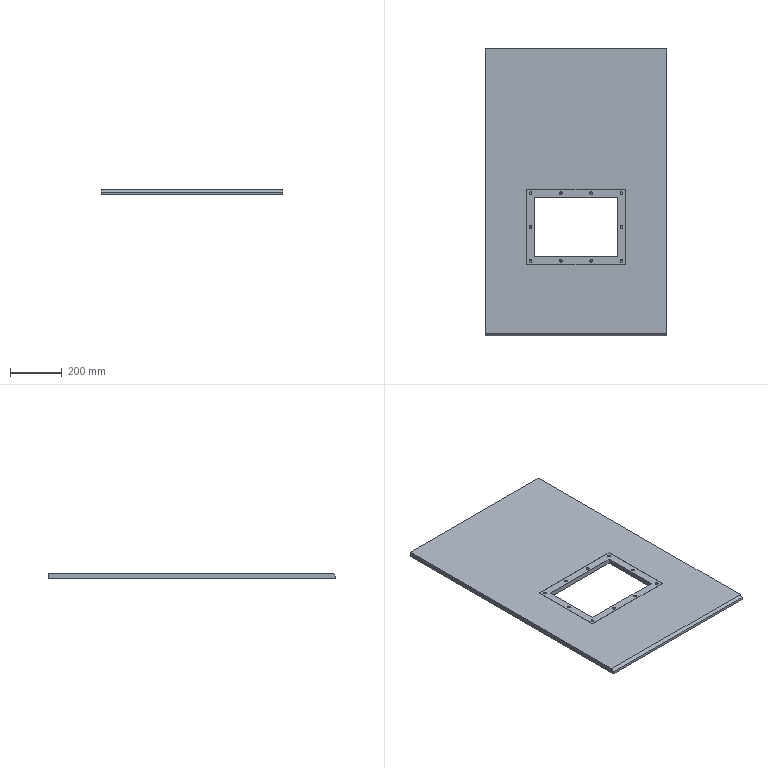Part | SolidWorks | features 3DProfileFeature 1, Chamfer 1, Extrusion 1, HoleWzd 1, ICE 1 | 1 solid | 56 faces | box 700 x 1110 x 20 mm | volume 13982805 mm3 | cylinder 20 | cone 20 | plane 16 | commonest cylinder face diameters 10.716 x20
STEP:
#1=CARTESIAN_POINT('',(169.642,550.,5.));
#2=VERTEX_POINT('',#1);
#3=CARTESIAN_POINT('',(180.358,550.,5.));
#4=VERTEX_POINT('',#3);
#5=CARTESIAN_POINT('',(175.,550.,5.));
#6=DIRECTION('',(0.,0.,1.));
#7=DIRECTION('',(1.,0.,0.));
#8=AXIS2_PLACEMENT_3D('',#5,#6,#7);
#9=CIRCLE('',#8,5.358);
#10=EDGE_CURVE('',#2,#4,#9,.T.);
#11=ORIENTED_EDGE('',*,*,#10,.F.);
#12=CARTESIAN_POINT('',(169.642,550.,19.));
#13=VERTEX_POINT('',#12);
#14=CARTESIAN_POINT('',(169.642,550.,19.));
#15=DIRECTION('',(0.,0.,1.));
#16=VECTOR('',#15,1000.);
#17=LINE('',#14,#16);
#18=EDGE_CURVE('',#2,#13,#17,.T.);
#19=ORIENTED_EDGE('',*,*,#18,.T.);
#20=CARTESIAN_POINT('',(180.358,550.,19.));
#21=VERTEX_POINT('',#20);
#22=CARTESIAN_POINT('',(175.,550.,19.));
#23=DIRECTION('',(0.,0.,1.));
#24=DIRECTION('',(1.,0.,0.));
#25=AXIS2_PLACEMENT_3D('',#22,#23,#24);
#26=CIRCLE('',#25,5.358);
#27=EDGE_CURVE('',#13,#21,#26,.T.);
#28=ORIENTED_EDGE('',*,*,#27,.T.);
#29=CARTESIAN_POINT('',(180.358,550.,19.));
#30=DIRECTION('',(0.,0.,1.));
#31=VECTOR('',#30,1000.);
#32=LINE('',#29,#31);
#33=EDGE_CURVE('',#4,#21,#32,.T.);
#34=ORIENTED_EDGE('',*,*,#33,.F.);
#35=EDGE_LOOP('',(#11,#19,#28,#34));
#36=FACE_OUTER_BOUND('',#35,.T.);
#37=CARTESIAN_POINT('',(175.,550.,19.));
#38=DIRECTION('',(0.,0.,1.));
#39=DIRECTION('',(1.,0.,0.));
#40=AXIS2_PLACEMENT_3D('',#37,#38,#39);
#41=CYLINDRICAL_SURFACE('',#40,5.358);
#42=ADVANCED_FACE('',(#36),#41,.F.);
#43=CARTESIAN_POINT('',(175.,550.,1.781));
#44=VERTEX_POINT('',#43);
#45=CARTESIAN_POINT('',(180.358,550.,5.));
#46=DIRECTION('',(0.8572,0.,0.515));
#47=VECTOR('',#46,1000.);
#48=LINE('',#45,#47);
#49=EDGE_CURVE('',#44,#4,#48,.T.);
#50=ORIENTED_EDGE('',*,*,#49,.F.);
#51=CARTESIAN_POINT('',(169.642,550.,5.));
#52=DIRECTION('',(-0.8572,0.,0.515));
#53=VECTOR('',#52,1000.);
#54=LINE('',#51,#53);
#55=EDGE_CURVE('',#44,#2,#54,.T.);
#56=ORIENTED_EDGE('',*,*,#55,.T.);
#57=ORIENTED_EDGE('',*,*,#10,.T.);
#58=EDGE_LOOP('',(#50,#56,#57));
#59=FACE_OUTER_BOUND('',#58,.T.);
#60=CARTESIAN_POINT('',(175.,550.,5.));
#61=DIRECTION('',(0.,0.,1.));
#62=DIRECTION('',(1.,0.,0.));
#63=AXIS2_PLACEMENT_3D('',#60,#61,#62);
#64=CONICAL_SURFACE('',#63,5.358,1.03);
#65=ADVANCED_FACE('',(#59),#64,.F.);
#66=CARTESIAN_POINT('',(286.142,550.,5.));
#67=VERTEX_POINT('',#66);
#68=CARTESIAN_POINT('',(296.858,550.,5.));
#69=VERTEX_POINT('',#68);
#70=CARTESIAN_POINT('',(291.5,550.,5.));
#71=DIRECTION('',(0.,0.,1.));
#72=DIRECTION('',(1.,0.,0.));
#73=AXIS2_PLACEMENT_3D('',#70,#71,#72);
#74=CIRCLE('',#73,5.358);
#75=EDGE_CURVE('',#67,#69,#74,.T.);
#76=ORIENTED_EDGE('',*,*,#75,.F.);
#77=CARTESIAN_POINT('',(286.142,550.,19.));
#78=VERTEX_POINT('',#77);
#79=CARTESIAN_POINT('',(286.142,550.,19.));
#80=DIRECTION('',(0.,0.,1.));
#81=VECTOR('',#80,1000.);
#82=LINE('',#79,#81);
#83=EDGE_CURVE('',#67,#78,#82,.T.);
#84=ORIENTED_EDGE('',*,*,#83,.T.);
#85=CARTESIAN_POINT('',(296.858,550.,19.));
#86=VERTEX_POINT('',#85);
#87=CARTESIAN_POINT('',(291.5,550.,19.));
#88=DIRECTION('',(0.,0.,1.));
#89=DIRECTION('',(1.,0.,0.));
#90=AXIS2_PLACEMENT_3D('',#87,#88,#89);
#91=CIRCLE('',#90,5.358);
#92=EDGE_CURVE('',#78,#86,#91,.T.);
#93=ORIENTED_EDGE('',*,*,#92,.T.);
#94=CARTESIAN_POINT('',(296.858,550.,19.));
#95=DIRECTION('',(0.,0.,1.));
#96=VECTOR('',#95,1000.);
#97=LINE('',#94,#96);
#98=EDGE_CURVE('',#69,#86,#97,.T.);
#99=ORIENTED_EDGE('',*,*,#98,.F.);
#100=EDGE_LOOP('',(#76,#84,#93,#99));
#101=FACE_OUTER_BOUND('',#100,.T.);
#102=CARTESIAN_POINT('',(291.5,550.,19.));
#103=DIRECTION('',(0.,0.,1.));
#104=DIRECTION('',(1.,0.,0.));
#105=AXIS2_PLACEMENT_3D('',#102,#103,#104);
#106=CYLINDRICAL_SURFACE('',#105,5.358);
#107=ADVANCED_FACE('',(#101),#106,.F.);
#108=CARTESIAN_POINT('',(291.5,550.,1.781));
#109=VERTEX_POINT('',#108);
#110=CARTESIAN_POINT('',(296.858,550.,5.));
#111=DIRECTION('',(0.8572,0.,0.515));
#112=VECTOR('',#111,1000.);
#113=LINE('',#110,#112);
#114=EDGE_CURVE('',#109,#69,#113,.T.);
#115=ORIENTED_EDGE('',*,*,#114,.F.);
#116=CARTESIAN_POINT('',(286.142,550.,5.));
#117=DIRECTION('',(-0.8572,0.,0.515));
#118=VECTOR('',#117,1000.);
#119=LINE('',#116,#118);
#120=EDGE_CURVE('',#109,#67,#119,.T.);
#121=ORIENTED_EDGE('',*,*,#120,.T.);
#122=ORIENTED_EDGE('',*,*,#75,.T.);
#123=EDGE_LOOP('',(#115,#121,#122));
#124=FACE_OUTER_BOUND('',#123,.T.);
#125=CARTESIAN_POINT('',(291.5,550.,5.));
#126=DIRECTION('',(0.,0.,1.));
#127=DIRECTION('',(1.,0.,0.));
#128=AXIS2_PLACEMENT_3D('',#125,#126,#127);
#129=CONICAL_SURFACE('',#128,5.358,1.03);
#130=ADVANCED_FACE('',(#124),#129,.F.);
#131=CARTESIAN_POINT('',(403.142,550.,5.));
#132=VERTEX_POINT('',#131);
#133=CARTESIAN_POINT('',(413.858,550.,5.));
#134=VERTEX_POINT('',#133);
#135=CARTESIAN_POINT('',(408.5,550.,5.));
#136=DIRECTION('',(0.,0.,1.));
#137=DIRECTION('',(1.,0.,0.));
#138=AXIS2_PLACEMENT_3D('',#135,#136,#137);
#139=CIRCLE('',#138,5.358);
#140=EDGE_CURVE('',#132,#134,#139,.T.);
#141=ORIENTED_EDGE('',*,*,#140,.F.);
#142=CARTESIAN_POINT('',(403.142,550.,19.));
#143=VERTEX_POINT('',#142);
#144=CARTESIAN_POINT('',(403.142,550.,19.));
#145=DIRECTION('',(0.,0.,1.));
#146=VECTOR('',#145,1000.);
#147=LINE('',#144,#146);
#148=EDGE_CURVE('',#132,#143,#147,.T.);
#149=ORIENTED_EDGE('',*,*,#148,.T.);
#150=CARTESIAN_POINT('',(413.858,550.,19.));
#151=VERTEX_POINT('',#150);
#152=CARTESIAN_POINT('',(408.5,550.,19.));
#153=DIRECTION('',(0.,0.,1.));
#154=DIRECTION('',(1.,0.,0.));
#155=AXIS2_PLACEMENT_3D('',#152,#153,#154);
#156=CIRCLE('',#155,5.358);
#157=EDGE_CURVE('',#143,#151,#156,.T.);
#158=ORIENTED_EDGE('',*,*,#157,.T.);
#159=CARTESIAN_POINT('',(413.858,550.,19.));
#160=DIRECTION('',(0.,0.,1.));
#161=VECTOR('',#160,1000.);
#162=LINE('',#159,#161);
#163=EDGE_CURVE('',#134,#151,#162,.T.);
#164=ORIENTED_EDGE('',*,*,#163,.F.);
#165=EDGE_LOOP('',(#141,#149,#158,#164));
#166=FACE_OUTER_BOUND('',#165,.T.);
#167=CARTESIAN_POINT('',(408.5,550.,19.));
#168=DIRECTION('',(0.,0.,1.));
#169=DIRECTION('',(1.,0.,0.));
#170=AXIS2_PLACEMENT_3D('',#167,#168,#169);
#171=CYLINDRICAL_SURFACE('',#170,5.358);
#172=ADVANCED_FACE('',(#166),#171,.F.);
#173=CARTESIAN_POINT('',(408.5,550.,1.781));
#174=VERTEX_POINT('',#173);
#175=CARTESIAN_POINT('',(413.858,550.,5.));
#176=DIRECTION('',(0.8572,0.,0.515));
#177=VECTOR('',#176,1000.);
#178=LINE('',#175,#177);
#179=EDGE_CURVE('',#174,#134,#178,.T.);
#180=ORIENTED_EDGE('',*,*,#179,.F.);
#181=CARTESIAN_POINT('',(403.142,550.,5.));
#182=DIRECTION('',(-0.8572,0.,0.515));
#183=VECTOR('',#182,1000.);
#184=LINE('',#181,#183);
#185=EDGE_CURVE('',#174,#132,#184,.T.);
#186=ORIENTED_EDGE('',*,*,#185,.T.);
#187=ORIENTED_EDGE('',*,*,#140,.T.);
#188=EDGE_LOOP('',(#180,#186,#187));
#189=FACE_OUTER_BOUND('',#188,.T.);
#190=CARTESIAN_POINT('',(408.5,550.,5.));
#191=DIRECTION('',(0.,0.,1.));
#192=DIRECTION('',(1.,0.,0.));
#193=AXIS2_PLACEMENT_3D('',#190,#191,#192);
#194=CONICAL_SURFACE('',#193,5.358,1.03);
#195=ADVANCED_FACE('',(#189),#194,.F.);
#196=CARTESIAN_POINT('',(519.642,550.,5.));
#197=VERTEX_POINT('',#196);
#198=CARTESIAN_POINT('',(530.358,550.,5.));
#199=VERTEX_POINT('',#198);
#200=CARTESIAN_POINT('',(525.,550.,5.));
#201=DIRECTION('',(0.,0.,1.));
#202=DIRECTION('',(1.,0.,0.));
#203=AXIS2_PLACEMENT_3D('',#200,#201,#202);
#204=CIRCLE('',#203,5.358);
#205=EDGE_CURVE('',#197,#199,#204,.T.);
#206=ORIENTED_EDGE('',*,*,#205,.F.);
#207=CARTESIAN_POINT('',(519.642,550.,19.));
#208=VERTEX_POINT('',#207);
#209=CARTESIAN_POINT('',(519.642,550.,19.));
#210=DIRECTION('',(0.,0.,1.));
#211=VECTOR('',#210,1000.);
#212=LINE('',#209,#211);
#213=EDGE_CURVE('',#197,#208,#212,.T.);
#214=ORIENTED_EDGE('',*,*,#213,.T.);
#215=CARTESIAN_POINT('',(530.358,550.,19.));
#216=VERTEX_POINT('',#215);
#217=CARTESIAN_POINT('',(525.,550.,19.));
#218=DIRECTION('',(0.,0.,1.));
#219=DIRECTION('',(1.,0.,0.));
#220=AXIS2_PLACEMENT_3D('',#217,#218,#219);
#221=CIRCLE('',#220,5.358);
#222=EDGE_CURVE('',#208,#216,#221,.T.);
#223=ORIENTED_EDGE('',*,*,#222,.T.);
#224=CARTESIAN_POINT('',(530.358,550.,19.));
#225=DIRECTION('',(0.,0.,1.));
#226=VECTOR('',#225,1000.);
#227=LINE('',#224,#226);
#228=EDGE_CURVE('',#199,#216,#227,.T.);
#229=ORIENTED_EDGE('',*,*,#228,.F.);
#230=EDGE_LOOP('',(#206,#214,#223,#229));
#231=FACE_OUTER_BOUND('',#230,.T.);
#232=CARTESIAN_POINT('',(525.,550.,19.));
#233=DIRECTION('',(0.,0.,1.));
#234=DIRECTION('',(1.,0.,0.));
#235=AXIS2_PLACEMENT_3D('',#232,#233,#234);
#236=CYLINDRICAL_SURFACE('',#235,5.358);
#237=ADVANCED_FACE('',(#231),#236,.F.);
#238=CARTESIAN_POINT('',(525.,550.,1.781));
#239=VERTEX_POINT('',#238);
#240=CARTESIAN_POINT('',(530.358,550.,5.));
#241=DIRECTION('',(0.8572,0.,0.515));
#242=VECTOR('',#241,1000.);
#243=LINE('',#240,#242);
#244=EDGE_CURVE('',#239,#199,#243,.T.);
#245=ORIENTED_EDGE('',*,*,#244,.F.);
#246=CARTESIAN_POINT('',(519.642,550.,5.));
#247=DIRECTION('',(-0.8572,0.,0.515));
#248=VECTOR('',#247,1000.);
#249=LINE('',#246,#248);
#250=EDGE_CURVE('',#239,#197,#249,.T.);
#251=ORIENTED_EDGE('',*,*,#250,.T.);
#252=ORIENTED_EDGE('',*,*,#205,.T.);
#253=EDGE_LOOP('',(#245,#251,#252));
#254=FACE_OUTER_BOUND('',#253,.T.);
#255=CARTESIAN_POINT('',(525.,550.,5.));
#256=DIRECTION('',(0.,0.,1.));
#257=DIRECTION('',(1.,0.,0.));
#258=AXIS2_PLACEMENT_3D('',#255,#256,#257);
#259=CONICAL_SURFACE('',#258,5.358,1.03);
#260=ADVANCED_FACE('',(#254),#259,.F.);
#261=CARTESIAN_POINT('',(519.642,420.,5.));
#262=VERTEX_POINT('',#261);
#263=CARTESIAN_POINT('',(530.358,420.,5.));
#264=VERTEX_POINT('',#263);
#265=CARTESIAN_POINT('',(525.,420.,5.));
#266=DIRECTION('',(0.,0.,1.));
#267=DIRECTION('',(1.,0.,0.));
#268=AXIS2_PLACEMENT_3D('',#265,#266,#267);
#269=CIRCLE('',#268,5.358);
#270=EDGE_CURVE('',#262,#264,#269,.T.);
#271=ORIENTED_EDGE('',*,*,#270,.F.);
#272=CARTESIAN_POINT('',(519.642,420.,19.));
#273=VERTEX_POINT('',#272);
#274=CARTESIAN_POINT('',(519.642,420.,19.));
#275=DIRECTION('',(0.,0.,1.));
#276=VECTOR('',#275,1000.);
#277=LINE('',#274,#276);
#278=EDGE_CURVE('',#262,#273,#277,.T.);
#279=ORIENTED_EDGE('',*,*,#278,.T.);
#280=CARTESIAN_POINT('',(530.358,420.,19.));
#281=VERTEX_POINT('',#280);
#282=CARTESIAN_POINT('',(525.,420.,19.));
#283=DIRECTION('',(0.,0.,1.));
#284=DIRECTION('',(1.,0.,0.));
#285=AXIS2_PLACEMENT_3D('',#282,#283,#284);
#286=CIRCLE('',#285,5.358);
#287=EDGE_CURVE('',#273,#281,#286,.T.);
#288=ORIENTED_EDGE('',*,*,#287,.T.);
#289=CARTESIAN_POINT('',(530.358,420.,19.));
#290=DIRECTION('',(0.,0.,1.));
#291=VECTOR('',#290,1000.);
#292=LINE('',#289,#291);
#293=EDGE_CURVE('',#264,#281,#292,.T.);
#294=ORIENTED_EDGE('',*,*,#293,.F.);
#295=EDGE_LOOP('',(#271,#279,#288,#294));
#296=FACE_OUTER_BOUND('',#295,.T.);
#297=CARTESIAN_POINT('',(525.,420.,19.));
#298=DIRECTION('',(0.,0.,1.));
#299=DIRECTION('',(1.,0.,0.));
#300=AXIS2_PLACEMENT_3D('',#297,#298,#299);
#301=CYLINDRICAL_SURFACE('',#300,5.358);
#302=ADVANCED_FACE('',(#296),#301,.F.);
#303=CARTESIAN_POINT('',(525.,420.,1.781));
#304=VERTEX_POINT('',#303);
#305=CARTESIAN_POINT('',(530.358,420.,5.));
#306=DIRECTION('',(0.8572,0.,0.515));
#307=VECTOR('',#306,1000.);
#308=LINE('',#305,#307);
#309=EDGE_CURVE('',#304,#264,#308,.T.);
#310=ORIENTED_EDGE('',*,*,#309,.F.);
#311=CARTESIAN_POINT('',(519.642,420.,5.));
#312=DIRECTION('',(-0.8572,0.,0.515));
#313=VECTOR('',#312,1000.);
#314=LINE('',#311,#313);
#315=EDGE_CURVE('',#304,#262,#314,.T.);
#316=ORIENTED_EDGE('',*,*,#315,.T.);
#317=ORIENTED_EDGE('',*,*,#270,.T.);
#318=EDGE_LOOP('',(#310,#316,#317));
#319=FACE_OUTER_BOUND('',#318,.T.);
#320=CARTESIAN_POINT('',(525.,420.,5.));
#321=DIRECTION('',(0.,0.,1.));
#322=DIRECTION('',(1.,0.,0.));
#323=AXIS2_PLACEMENT_3D('',#320,#321,#322);
#324=CONICAL_SURFACE('',#323,5.358,1.03);
#325=ADVANCED_FACE('',(#319),#324,.F.);
#326=CARTESIAN_POINT('',(519.642,290.,5.));
#327=VERTEX_POINT('',#326);
#328=CARTESIAN_POINT('',(530.358,290.,5.));
#329=VERTEX_POINT('',#328);
#330=CARTESIAN_POINT('',(525.,290.,5.));
#331=DIRECTION('',(0.,0.,1.));
#332=DIRECTION('',(1.,0.,0.));
#333=AXIS2_PLACEMENT_3D('',#330,#331,#332);
#334=CIRCLE('',#333,5.358);
#335=EDGE_CURVE('',#327,#329,#334,.T.);
#336=ORIENTED_EDGE('',*,*,#335,.F.);
#337=CARTESIAN_POINT('',(519.642,290.,19.));
#338=VERTEX_POINT('',#337);
#339=CARTESIAN_POINT('',(519.642,290.,19.));
#340=DIRECTION('',(0.,0.,1.));
#341=VECTOR('',#340,1000.);
#342=LINE('',#339,#341);
#343=EDGE_CURVE('',#327,#338,#342,.T.);
#344=ORIENTED_EDGE('',*,*,#343,.T.);
#345=CARTESIAN_POINT('',(530.358,290.,19.));
#346=VERTEX_POINT('',#345);
#347=CARTESIAN_POINT('',(525.,290.,19.));
#348=DIRECTION('',(0.,0.,1.));
#349=DIRECTION('',(1.,0.,0.));
#350=AXIS2_PLACEMENT_3D('',#347,#348,#349);
#351=CIRCLE('',#350,5.358);
#352=EDGE_CURVE('',#338,#346,#351,.T.);
#353=ORIENTED_EDGE('',*,*,#352,.T.);
#354=CARTESIAN_POINT('',(530.358,290.,19.));
#355=DIRECTION('',(0.,0.,1.));
#356=VECTOR('',#355,1000.);
#357=LINE('',#354,#356);
#358=EDGE_CURVE('',#329,#346,#357,.T.);
#359=ORIENTED_EDGE('',*,*,#358,.F.);
#360=EDGE_LOOP('',(#336,#344,#353,#359));
#361=FACE_OUTER_BOUND('',#360,.T.);
#362=CARTESIAN_POINT('',(525.,290.,19.));
#363=DIRECTION('',(0.,0.,1.));
#364=DIRECTION('',(1.,0.,0.));
#365=AXIS2_PLACEMENT_3D('',#362,#363,#364);
#366=CYLINDRICAL_SURFACE('',#365,5.358);
#367=ADVANCED_FACE('',(#361),#366,.F.);
#368=CARTESIAN_POINT('',(525.,290.,1.781));
#369=VERTEX_POINT('',#368);
#370=CARTESIAN_POINT('',(530.358,290.,5.));
#371=DIRECTION('',(0.8572,0.,0.515));
#372=VECTOR('',#371,1000.);
#373=LINE('',#370,#372);
#374=EDGE_CURVE('',#369,#329,#373,.T.);
#375=ORIENTED_EDGE('',*,*,#374,.F.);
#376=CARTESIAN_POINT('',(519.642,290.,5.));
#377=DIRECTION('',(-0.8572,0.,0.515));
#378=VECTOR('',#377,1000.);
#379=LINE('',#376,#378);
#380=EDGE_CURVE('',#369,#327,#379,.T.);
#381=ORIENTED_EDGE('',*,*,#380,.T.);
#382=ORIENTED_EDGE('',*,*,#335,.T.);
#383=EDGE_LOOP('',(#375,#381,#382));
#384=FACE_OUTER_BOUND('',#383,.T.);
#385=CARTESIAN_POINT('',(525.,290.,5.));
#386=DIRECTION('',(0.,0.,1.));
#387=DIRECTION('',(1.,0.,0.));
#388=AXIS2_PLACEMENT_3D('',#385,#386,#387);
#389=CONICAL_SURFACE('',#388,5.358,1.03);
#390=ADVANCED_FACE('',(#384),#389,.F.);
#391=CARTESIAN_POINT('',(403.142,290.,5.));
#392=VERTEX_POINT('',#391);
#393=CARTESIAN_POINT('',(413.858,290.,5.));
#394=VERTEX_POINT('',#393);
#395=CARTESIAN_POINT('',(408.5,290.,5.));
#396=DIRECTION('',(0.,0.,1.));
#397=DIRECTION('',(1.,0.,0.));
#398=AXIS2_PLACEMENT_3D('',#395,#396,#397);
#399=CIRCLE('',#398,5.358);
#400=EDGE_CURVE('',#392,#394,#399,.T.);
#401=ORIENTED_EDGE('',*,*,#400,.F.);
#402=CARTESIAN_POINT('',(403.142,290.,19.));
#403=VERTEX_POINT('',#402);
#404=CARTESIAN_POINT('',(403.142,290.,19.));
#405=DIRECTION('',(0.,0.,1.));
#406=VECTOR('',#405,1000.);
#407=LINE('',#404,#406);
#408=EDGE_CURVE('',#392,#403,#407,.T.);
#409=ORIENTED_EDGE('',*,*,#408,.T.);
#410=CARTESIAN_POINT('',(413.858,290.,19.));
#411=VERTEX_POINT('',#410);
#412=CARTESIAN_POINT('',(408.5,290.,19.));
#413=DIRECTION('',(0.,0.,1.));
#414=DIRECTION('',(1.,0.,0.));
#415=AXIS2_PLACEMENT_3D('',#412,#413,#414);
#416=CIRCLE('',#415,5.358);
#417=EDGE_CURVE('',#403,#411,#416,.T.);
#418=ORIENTED_EDGE('',*,*,#417,.T.);
#419=CARTESIAN_POINT('',(413.858,290.,19.));
#420=DIRECTION('',(0.,0.,1.));
#421=VECTOR('',#420,1000.);
#422=LINE('',#419,#421);
#423=EDGE_CURVE('',#394,#411,#422,.T.);
#424=ORIENTED_EDGE('',*,*,#423,.F.);
#425=EDGE_LOOP('',(#401,#409,#418,#424));
#426=FACE_OUTER_BOUND('',#425,.T.);
#427=CARTESIAN_POINT('',(408.5,290.,19.));
#428=DIRECTION('',(0.,0.,1.));
#429=DIRECTION('',(1.,0.,0.));
#430=AXIS2_PLACEMENT_3D('',#427,#428,#429);
#431=CYLINDRICAL_SURFACE('',#430,5.358);
#432=ADVANCED_FACE('',(#426),#431,.F.);
#433=CARTESIAN_POINT('',(408.5,290.,1.781));
#434=VERTEX_POINT('',#433);
#435=CARTESIAN_POINT('',(413.858,290.,5.));
#436=DIRECTION('',(0.8572,0.,0.515));
#437=VECTOR('',#436,1000.);
#438=LINE('',#435,#437);
#439=EDGE_CURVE('',#434,#394,#438,.T.);
#440=ORIENTED_EDGE('',*,*,#439,.F.);
#441=CARTESIAN_POINT('',(403.142,290.,5.));
#442=DIRECTION('',(-0.8572,0.,0.515));
#443=VECTOR('',#442,1000.);
#444=LINE('',#441,#443);
#445=EDGE_CURVE('',#434,#392,#444,.T.);
#446=ORIENTED_EDGE('',*,*,#445,.T.);
#447=ORIENTED_EDGE('',*,*,#400,.T.);
#448=EDGE_LOOP('',(#440,#446,#447));
#449=FACE_OUTER_BOUND('',#448,.T.);
#450=CARTESIAN_POINT('',(408.5,290.,5.));
#451=DIRECTION('',(0.,0.,1.));
#452=DIRECTION('',(1.,0.,0.));
#453=AXIS2_PLACEMENT_3D('',#450,#451,#452);
#454=CONICAL_SURFACE('',#453,5.358,1.03);
#455=ADVANCED_FACE('',(#449),#454,.F.);
#456=CARTESIAN_POINT('',(286.142,290.,5.));
#457=VERTEX_POINT('',#456);
#458=CARTESIAN_POINT('',(296.858,290.,5.));
#459=VERTEX_POINT('',#458);
#460=CARTESIAN_POINT('',(291.5,290.,5.));
#461=DIRECTION('',(0.,0.,1.));
#462=DIRECTION('',(1.,0.,0.));
#463=AXIS2_PLACEMENT_3D('',#460,#461,#462);
#464=CIRCLE('',#463,5.358);
#465=EDGE_CURVE('',#457,#459,#464,.T.);
#466=ORIENTED_EDGE('',*,*,#465,.F.);
#467=CARTESIAN_POINT('',(286.142,290.,19.));
#468=VERTEX_POINT('',#467);
#469=CARTESIAN_POINT('',(286.142,290.,19.));
#470=DIRECTION('',(0.,0.,1.));
#471=VECTOR('',#470,1000.);
#472=LINE('',#469,#471);
#473=EDGE_CURVE('',#457,#468,#472,.T.);
#474=ORIENTED_EDGE('',*,*,#473,.T.);
#475=CARTESIAN_POINT('',(296.858,290.,19.));
#476=VERTEX_POINT('',#475);
#477=CARTESIAN_POINT('',(291.5,290.,19.));
#478=DIRECTION('',(0.,0.,1.));
#479=DIRECTION('',(1.,0.,0.));
#480=AXIS2_PLACEMENT_3D('',#477,#478,#479);
#481=CIRCLE('',#480,5.358);
#482=EDGE_CURVE('',#468,#476,#481,.T.);
#483=ORIENTED_EDGE('',*,*,#482,.T.);
#484=CARTESIAN_POINT('',(296.858,290.,19.));
#485=DIRECTION('',(0.,0.,1.));
#486=VECTOR('',#485,1000.);
#487=LINE('',#484,#486);
#488=EDGE_CURVE('',#459,#476,#487,.T.);
#489=ORIENTED_EDGE('',*,*,#488,.F.);
#490=EDGE_LOOP('',(#466,#474,#483,#489));
#491=FACE_OUTER_BOUND('',#490,.T.);
#492=CARTESIAN_POINT('',(291.5,290.,19.));
#493=DIRECTION('',(0.,0.,1.));
#494=DIRECTION('',(1.,0.,0.));
#495=AXIS2_PLACEMENT_3D('',#492,#493,#494);
#496=CYLINDRICAL_SURFACE('',#495,5.358);
#497=ADVANCED_FACE('',(#491),#496,.F.);
#498=CARTESIAN_POINT('',(291.5,290.,1.781));
#499=VERTEX_POINT('',#498);
#500=CARTESIAN_POINT('',(296.858,290.,5.));
#501=DIRECTION('',(0.8572,0.,0.515));
#502=VECTOR('',#501,1000.);
#503=LINE('',#500,#502);
#504=EDGE_CURVE('',#499,#459,#503,.T.);
#505=ORIENTED_EDGE('',*,*,#504,.F.);
#506=CARTESIAN_POINT('',(286.142,290.,5.));
#507=DIRECTION('',(-0.8572,0.,0.515));
#508=VECTOR('',#507,1000.);
#509=LINE('',#506,#508);
#510=EDGE_CURVE('',#499,#457,#509,.T.);
#511=ORIENTED_EDGE('',*,*,#510,.T.);
#512=ORIENTED_EDGE('',*,*,#465,.T.);
#513=EDGE_LOOP('',(#505,#511,#512));
#514=FACE_OUTER_BOUND('',#513,.T.);
#515=CARTESIAN_POINT('',(291.5,290.,5.));
#516=DIRECTION('',(0.,0.,1.));
#517=DIRECTION('',(1.,0.,0.));
#518=AXIS2_PLACEMENT_3D('',#515,#516,#517);
#519=CONICAL_SURFACE('',#518,5.358,1.03);
#520=ADVANCED_FACE('',(#514),#519,.F.);
#521=CARTESIAN_POINT('',(169.642,290.,5.));
#522=VERTEX_POINT('',#521);
#523=CARTESIAN_POINT('',(180.358,290.,5.));
#524=VERTEX_POINT('',#523);
#525=CARTESIAN_POINT('',(175.,290.,5.));
#526=DIRECTION('',(0.,0.,1.));
#527=DIRECTION('',(1.,0.,0.));
#528=AXIS2_PLACEMENT_3D('',#525,#526,#527);
#529=CIRCLE('',#528,5.358);
#530=EDGE_CURVE('',#522,#524,#529,.T.);
#531=ORIENTED_EDGE('',*,*,#530,.F.);
#532=CARTESIAN_POINT('',(169.642,290.,19.));
#533=VERTEX_POINT('',#532);
#534=CARTESIAN_POINT('',(169.642,290.,19.));
#535=DIRECTION('',(0.,0.,1.));
#536=VECTOR('',#535,1000.);
#537=LINE('',#534,#536);
#538=EDGE_CURVE('',#522,#533,#537,.T.);
#539=ORIENTED_EDGE('',*,*,#538,.T.);
#540=CARTESIAN_POINT('',(180.358,290.,19.));
#541=VERTEX_POINT('',#540);
#542=CARTESIAN_POINT('',(175.,290.,19.));
#543=DIRECTION('',(0.,0.,1.));
#544=DIRECTION('',(1.,0.,0.));
#545=AXIS2_PLACEMENT_3D('',#542,#543,#544);
#546=CIRCLE('',#545,5.358);
#547=EDGE_CURVE('',#533,#541,#546,.T.);
#548=ORIENTED_EDGE('',*,*,#547,.T.);
#549=CARTESIAN_POINT('',(180.358,290.,19.));
#550=DIRECTION('',(0.,0.,1.));
#551=VECTOR('',#550,1000.);
#552=LINE('',#549,#551);
#553=EDGE_CURVE('',#524,#541,#552,.T.);
#554=ORIENTED_EDGE('',*,*,#553,.F.);
#555=EDGE_LOOP('',(#531,#539,#548,#554));
#556=FACE_OUTER_BOUND('',#555,.T.);
#557=CARTESIAN_POINT('',(175.,290.,19.));
#558=DIRECTION('',(0.,0.,1.));
#559=DIRECTION('',(1.,0.,0.));
#560=AXIS2_PLACEMENT_3D('',#557,#558,#559);
#561=CYLINDRICAL_SURFACE('',#560,5.358);
#562=ADVANCED_FACE('',(#556),#561,.F.);
#563=CARTESIAN_POINT('',(175.,290.,1.781));
#564=VERTEX_POINT('',#563);
#565=CARTESIAN_POINT('',(180.358,290.,5.));
#566=DIRECTION('',(0.8572,0.,0.515));
#567=VECTOR('',#566,1000.);
#568=LINE('',#565,#567);
#569=EDGE_CURVE('',#564,#524,#568,.T.);
#570=ORIENTED_EDGE('',*,*,#569,.F.);
#571=CARTESIAN_POINT('',(169.642,290.,5.));
#572=DIRECTION('',(-0.8572,0.,0.515));
#573=VECTOR('',#572,1000.);
#574=LINE('',#571,#573);
#575=EDGE_CURVE('',#564,#522,#574,.T.);
#576=ORIENTED_EDGE('',*,*,#575,.T.);
#577=ORIENTED_EDGE('',*,*,#530,.T.);
#578=EDGE_LOOP('',(#570,#576,#577));
#579=FACE_OUTER_BOUND('',#578,.T.);
#580=CARTESIAN_POINT('',(175.,290.,5.));
#581=DIRECTION('',(0.,0.,1.));
#582=DIRECTION('',(1.,0.,0.));
#583=AXIS2_PLACEMENT_3D('',#580,#581,#582);
#584=CONICAL_SURFACE('',#583,5.358,1.03);
#585=ADVANCED_FACE('',(#579),#584,.F.);
#586=CARTESIAN_POINT('',(169.642,420.,5.));
#587=VERTEX_POINT('',#586);
#588=CARTESIAN_POINT('',(180.358,420.,5.));
#589=VERTEX_POINT('',#588);
#590=CARTESIAN_POINT('',(175.,420.,5.));
#591=DIRECTION('',(0.,0.,1.));
#592=DIRECTION('',(1.,0.,0.));
#593=AXIS2_PLACEMENT_3D('',#590,#591,#592);
#594=CIRCLE('',#593,5.358);
#595=EDGE_CURVE('',#587,#589,#594,.T.);
#596=ORIENTED_EDGE('',*,*,#595,.F.);
#597=CARTESIAN_POINT('',(169.642,420.,19.));
#598=VERTEX_POINT('',#597);
#599=CARTESIAN_POINT('',(169.642,420.,19.));
#600=DIRECTION('',(0.,0.,1.));
#601=VECTOR('',#600,1000.);
#602=LINE('',#599,#601);
#603=EDGE_CURVE('',#587,#598,#602,.T.);
#604=ORIENTED_EDGE('',*,*,#603,.T.);
#605=CARTESIAN_POINT('',(180.358,420.,19.));
#606=VERTEX_POINT('',#605);
#607=CARTESIAN_POINT('',(175.,420.,19.));
#608=DIRECTION('',(0.,0.,1.));
#609=DIRECTION('',(1.,0.,0.));
#610=AXIS2_PLACEMENT_3D('',#607,#608,#609);
#611=CIRCLE('',#610,5.358);
#612=EDGE_CURVE('',#598,#606,#611,.T.);
#613=ORIENTED_EDGE('',*,*,#612,.T.);
#614=CARTESIAN_POINT('',(180.358,420.,19.));
#615=DIRECTION('',(0.,0.,1.));
#616=VECTOR('',#615,1000.);
#617=LINE('',#614,#616);
#618=EDGE_CURVE('',#589,#606,#617,.T.);
#619=ORIENTED_EDGE('',*,*,#618,.F.);
#620=EDGE_LOOP('',(#596,#604,#613,#619));
#621=FACE_OUTER_BOUND('',#620,.T.);
#622=CARTESIAN_POINT('',(175.,420.,19.));
#623=DIRECTION('',(0.,0.,1.));
#624=DIRECTION('',(1.,0.,0.));
#625=AXIS2_PLACEMENT_3D('',#622,#623,#624);
#626=CYLINDRICAL_SURFACE('',#625,5.358);
#627=ADVANCED_FACE('',(#621),#626,.F.);
#628=CARTESIAN_POINT('',(175.,420.,1.781));
#629=VERTEX_POINT('',#628);
#630=CARTESIAN_POINT('',(180.358,420.,5.));
#631=DIRECTION('',(0.8572,0.,0.515));
#632=VECTOR('',#631,1000.);
#633=LINE('',#630,#632);
#634=EDGE_CURVE('',#629,#589,#633,.T.);
#635=ORIENTED_EDGE('',*,*,#634,.F.);
#636=CARTESIAN_POINT('',(169.642,420.,5.));
#637=DIRECTION('',(-0.8572,0.,0.515));
#638=VECTOR('',#637,1000.);
#639=LINE('',#636,#638);
#640=EDGE_CURVE('',#629,#587,#639,.T.);
#641=ORIENTED_EDGE('',*,*,#640,.T.);
#642=ORIENTED_EDGE('',*,*,#595,.T.);
#643=EDGE_LOOP('',(#635,#641,#642));
#644=FACE_OUTER_BOUND('',#643,.T.);
#645=CARTESIAN_POINT('',(175.,420.,5.));
#646=DIRECTION('',(0.,0.,1.));
#647=DIRECTION('',(1.,0.,0.));
#648=AXIS2_PLACEMENT_3D('',#645,#646,#647);
#649=CONICAL_SURFACE('',#648,5.358,1.03);
#650=ADVANCED_FACE('',(#644),#649,.F.);
#651=CARTESIAN_POINT('',(190.,535.,19.));
#652=VERTEX_POINT('',#651);
#653=CARTESIAN_POINT('',(190.,535.,0.));
#654=VERTEX_POINT('',#653);
#655=CARTESIAN_POINT('',(190.,535.,20.));
#656=DIRECTION('',(0.,0.,-1.));
#657=VECTOR('',#656,1000.);
#658=LINE('',#655,#657);
#659=EDGE_CURVE('',#652,#654,#658,.T.);
#660=ORIENTED_EDGE('',*,*,#659,.F.);
#661=CARTESIAN_POINT('',(190.,305.,19.));
#662=VERTEX_POINT('',#661);
#663=CARTESIAN_POINT('',(190.,535.,19.));
#664=DIRECTION('',(0.,-1.,0.));
#665=VECTOR('',#664,1000.);
#666=LINE('',#663,#665);
#667=EDGE_CURVE('',#652,#662,#666,.T.);
#668=ORIENTED_EDGE('',*,*,#667,.T.);
#669=CARTESIAN_POINT('',(190.,305.,0.));
#670=VERTEX_POINT('',#669);
#671=CARTESIAN_POINT('',(190.,305.,20.));
#672=DIRECTION('',(0.,0.,-1.));
#673=VECTOR('',#672,1000.);
#674=LINE('',#671,#673);
#675=EDGE_CURVE('',#662,#670,#674,.T.);
#676=ORIENTED_EDGE('',*,*,#675,.T.);
#677=CARTESIAN_POINT('',(190.,535.,0.));
#678=DIRECTION('',(0.,-1.,0.));
#679=VECTOR('',#678,1000.);
#680=LINE('',#677,#679);
#681=EDGE_CURVE('',#654,#670,#680,.T.);
#682=ORIENTED_EDGE('',*,*,#681,.F.);
#683=EDGE_LOOP('',(#660,#668,#676,#682));
#684=FACE_OUTER_BOUND('',#683,.T.);
#685=CARTESIAN_POINT('',(190.,535.,20.));
#686=DIRECTION('',(1.,0.,0.));
#687=DIRECTION('',(0.,0.,-1.));
#688=AXIS2_PLACEMENT_3D('',#685,#686,#687);
#689=PLANE('',#688);
#690=ADVANCED_FACE('',(#684),#689,.T.);
#691=ORIENTED_EDGE('',*,*,#675,.F.);
#692=CARTESIAN_POINT('',(510.,305.,19.));
#693=VERTEX_POINT('',#692);
#694=CARTESIAN_POINT('',(190.,305.,19.));
#695=DIRECTION('',(1.,0.,0.));
#696=VECTOR('',#695,1000.);
#697=LINE('',#694,#696);
#698=EDGE_CURVE('',#662,#693,#697,.T.);
#699=ORIENTED_EDGE('',*,*,#698,.T.);
#700=CARTESIAN_POINT('',(510.,305.,0.));
#701=VERTEX_POINT('',#700);
#702=CARTESIAN_POINT('',(510.,305.,20.));
#703=DIRECTION('',(0.,0.,-1.));
#704=VECTOR('',#703,1000.);
#705=LINE('',#702,#704);
#706=EDGE_CURVE('',#693,#701,#705,.T.);
#707=ORIENTED_EDGE('',*,*,#706,.T.);
#708=CARTESIAN_POINT('',(190.,305.,0.));
#709=DIRECTION('',(1.,0.,0.));
#710=VECTOR('',#709,1000.);
#711=LINE('',#708,#710);
#712=EDGE_CURVE('',#670,#701,#711,.T.);
#713=ORIENTED_EDGE('',*,*,#712,.F.);
#714=EDGE_LOOP('',(#691,#699,#707,#713));
#715=FACE_OUTER_BOUND('',#714,.T.);
#716=CARTESIAN_POINT('',(190.,305.,20.));
#717=DIRECTION('',(0.,1.,0.));
#718=DIRECTION('',(-1.,0.,0.));
#719=AXIS2_PLACEMENT_3D('',#716,#717,#718);
#720=PLANE('',#719);
#721=ADVANCED_FACE('',(#715),#720,.T.);
#722=ORIENTED_EDGE('',*,*,#706,.F.);
#723=CARTESIAN_POINT('',(510.,535.,19.));
#724=VERTEX_POINT('',#723);
#725=CARTESIAN_POINT('',(510.,535.,19.));
#726=DIRECTION('',(0.,1.,0.));
#727=VECTOR('',#726,1000.);
#728=LINE('',#725,#727);
#729=EDGE_CURVE('',#693,#724,#728,.T.);
#730=ORIENTED_EDGE('',*,*,#729,.T.);
#731=CARTESIAN_POINT('',(510.,535.,0.));
#732=VERTEX_POINT('',#731);
#733=CARTESIAN_POINT('',(510.,535.,20.));
#734=DIRECTION('',(0.,0.,-1.));
#735=VECTOR('',#734,1000.);
#736=LINE('',#733,#735);
#737=EDGE_CURVE('',#724,#732,#736,.T.);
#738=ORIENTED_EDGE('',*,*,#737,.T.);
#739=CARTESIAN_POINT('',(510.,535.,0.));
#740=DIRECTION('',(0.,1.,0.));
#741=VECTOR('',#740,1000.);
#742=LINE('',#739,#741);
#743=EDGE_CURVE('',#701,#732,#742,.T.);
#744=ORIENTED_EDGE('',*,*,#743,.F.);
#745=EDGE_LOOP('',(#722,#730,#738,#744));
#746=FACE_OUTER_BOUND('',#745,.T.);
#747=CARTESIAN_POINT('',(510.,535.,20.));
#748=DIRECTION('',(-1.,0.,0.));
#749=DIRECTION('',(0.,0.,1.));
#750=AXIS2_PLACEMENT_3D('',#747,#748,#749);
#751=PLANE('',#750);
#752=ADVANCED_FACE('',(#746),#751,.T.);
#753=ORIENTED_EDGE('',*,*,#737,.F.);
#754=CARTESIAN_POINT('',(190.,535.,19.));
#755=DIRECTION('',(-1.,0.,0.));
#756=VECTOR('',#755,1000.);
#757=LINE('',#754,#756);
#758=EDGE_CURVE('',#724,#652,#757,.T.);
#759=ORIENTED_EDGE('',*,*,#758,.T.);
#760=ORIENTED_EDGE('',*,*,#659,.T.);
#761=CARTESIAN_POINT('',(190.,535.,0.));
#762=DIRECTION('',(-1.,0.,0.));
#763=VECTOR('',#762,1000.);
#764=LINE('',#761,#763);
#765=EDGE_CURVE('',#732,#654,#764,.T.);
#766=ORIENTED_EDGE('',*,*,#765,.F.);
#767=EDGE_LOOP('',(#753,#759,#760,#766));
#768=FACE_OUTER_BOUND('',#767,.T.);
#769=CARTESIAN_POINT('',(190.,535.,20.));
#770=DIRECTION('',(0.,-1.,0.));
#771=DIRECTION('',(0.,0.,-1.));
#772=AXIS2_PLACEMENT_3D('',#769,#770,#771);
#773=PLANE('',#772);
#774=ADVANCED_FACE('',(#768),#773,.T.);
#775=CARTESIAN_POINT('',(160.,275.,20.));
#776=VERTEX_POINT('',#775);
#777=CARTESIAN_POINT('',(540.,275.,20.));
#778=VERTEX_POINT('',#777);
#779=CARTESIAN_POINT('',(160.,275.,20.));
#780=DIRECTION('',(1.,0.,0.));
#781=VECTOR('',#780,1000.);
#782=LINE('',#779,#781);
#783=EDGE_CURVE('',#776,#778,#782,.T.);
#784=ORIENTED_EDGE('',*,*,#783,.F.);
#785=CARTESIAN_POINT('',(160.,565.,20.));
#786=VERTEX_POINT('',#785);
#787=CARTESIAN_POINT('',(160.,565.,20.));
#788=DIRECTION('',(0.,-1.,0.));
#789=VECTOR('',#788,1000.);
#790=LINE('',#787,#789);
#791=EDGE_CURVE('',#786,#776,#790,.T.);
#792=ORIENTED_EDGE('',*,*,#791,.F.);
#793=CARTESIAN_POINT('',(540.,565.,20.));
#794=VERTEX_POINT('',#793);
#795=CARTESIAN_POINT('',(160.,565.,20.));
#796=DIRECTION('',(-1.,0.,0.));
#797=VECTOR('',#796,1000.);
#798=LINE('',#795,#797);
#799=EDGE_CURVE('',#794,#786,#798,.T.);
#800=ORIENTED_EDGE('',*,*,#799,.F.);
#801=CARTESIAN_POINT('',(540.,565.,20.));
#802=DIRECTION('',(0.,1.,0.));
#803=VECTOR('',#802,1000.);
#804=LINE('',#801,#803);
#805=EDGE_CURVE('',#778,#794,#804,.T.);
#806=ORIENTED_EDGE('',*,*,#805,.F.);
#807=EDGE_LOOP('',(#784,#792,#800,#806));
#808=FACE_BOUND('',#807,.T.);
#809=CARTESIAN_POINT('',(0.,1110.,20.));
#810=VERTEX_POINT('',#809);
#811=CARTESIAN_POINT('',(0.,10.,20.));
#812=VERTEX_POINT('',#811);
#813=CARTESIAN_POINT('',(0.,0.,20.));
#814=DIRECTION('',(0.,-1.,0.));
#815=VECTOR('',#814,1000.);
#816=LINE('',#813,#815);
#817=EDGE_CURVE('',#810,#812,#816,.T.);
#818=ORIENTED_EDGE('',*,*,#817,.T.);
#819=CARTESIAN_POINT('',(700.,10.,20.));
#820=VERTEX_POINT('',#819);
#821=CARTESIAN_POINT('',(0.,10.,20.));
#822=DIRECTION('',(1.,0.,0.));
#823=VECTOR('',#822,1000.);
#824=LINE('',#821,#823);
#825=EDGE_CURVE('',#812,#820,#824,.T.);
#826=ORIENTED_EDGE('',*,*,#825,.T.);
#827=CARTESIAN_POINT('',(700.,1110.,20.));
#828=VERTEX_POINT('',#827);
#829=CARTESIAN_POINT('',(700.,0.,20.));
#830=DIRECTION('',(0.,1.,0.));
#831=VECTOR('',#830,1000.);
#832=LINE('',#829,#831);
#833=EDGE_CURVE('',#820,#828,#832,.T.);
#834=ORIENTED_EDGE('',*,*,#833,.T.);
#835=CARTESIAN_POINT('',(0.,1110.,20.));
#836=DIRECTION('',(-1.,0.,0.));
#837=VECTOR('',#836,1000.);
#838=LINE('',#835,#837);
#839=EDGE_CURVE('',#828,#810,#838,.T.);
#840=ORIENTED_EDGE('',*,*,#839,.T.);
#841=EDGE_LOOP('',(#818,#826,#834,#840));
#842=FACE_OUTER_BOUND('',#841,.T.);
#843=CARTESIAN_POINT('',(0.,0.,20.));
#844=DIRECTION('',(0.,0.,-1.));
#845=DIRECTION('',(-1.,0.,0.));
#846=AXIS2_PLACEMENT_3D('',#843,#844,#845);
#847=PLANE('',#846);
#848=ADVANCED_FACE('',(#808,#842),#847,.F.);
#849=CARTESIAN_POINT('',(0.,1110.,0.));
#850=VERTEX_POINT('',#849);
#851=CARTESIAN_POINT('',(0.,0.,0.));
#852=VERTEX_POINT('',#851);
#853=CARTESIAN_POINT('',(0.,0.,0.));
#854=DIRECTION('',(0.,-1.,0.));
#855=VECTOR('',#854,1000.);
#856=LINE('',#853,#855);
#857=EDGE_CURVE('',#850,#852,#856,.T.);
#858=ORIENTED_EDGE('',*,*,#857,.F.);
#859=CARTESIAN_POINT('',(700.,1110.,0.));
#860=VERTEX_POINT('',#859);
#861=CARTESIAN_POINT('',(0.,1110.,0.));
#862=DIRECTION('',(-1.,0.,0.));
#863=VECTOR('',#862,1000.);
#864=LINE('',#861,#863);
#865=EDGE_CURVE('',#860,#850,#864,.T.);
#866=ORIENTED_EDGE('',*,*,#865,.F.);
#867=CARTESIAN_POINT('',(700.,0.,0.));
#868=VERTEX_POINT('',#867);
#869=CARTESIAN_POINT('',(700.,0.,0.));
#870=DIRECTION('',(0.,1.,0.));
#871=VECTOR('',#870,1000.);
#872=LINE('',#869,#871);
#873=EDGE_CURVE('',#868,#860,#872,.T.);
#874=ORIENTED_EDGE('',*,*,#873,.F.);
#875=CARTESIAN_POINT('',(0.,0.,0.));
#876=DIRECTION('',(1.,0.,0.));
#877=VECTOR('',#876,1000.);
#878=LINE('',#875,#877);
#879=EDGE_CURVE('',#852,#868,#878,.T.);
#880=ORIENTED_EDGE('',*,*,#879,.F.);
#881=EDGE_LOOP('',(#858,#866,#874,#880));
#882=FACE_OUTER_BOUND('',#881,.T.);
#883=ORIENTED_EDGE('',*,*,#765,.T.);
#884=ORIENTED_EDGE('',*,*,#681,.T.);
#885=ORIENTED_EDGE('',*,*,#712,.T.);
#886=ORIENTED_EDGE('',*,*,#743,.T.);
#887=EDGE_LOOP('',(#883,#884,#885,#886));
#888=FACE_BOUND('',#887,.T.);
#889=CARTESIAN_POINT('',(0.,0.,0.));
#890=DIRECTION('',(0.,0.,-1.));
#891=DIRECTION('',(-1.,0.,0.));
#892=AXIS2_PLACEMENT_3D('',#889,#890,#891);
#893=PLANE('',#892);
#894=ADVANCED_FACE('',(#882,#888),#893,.T.);
#895=CARTESIAN_POINT('',(0.,0.,10.));
#896=VERTEX_POINT('',#895);
#897=CARTESIAN_POINT('',(0.,0.,20.));
#898=DIRECTION('',(0.,0.,-1.));
#899=VECTOR('',#898,1000.);
#900=LINE('',#897,#899);
#901=EDGE_CURVE('',#896,#852,#900,.T.);
#902=ORIENTED_EDGE('',*,*,#901,.F.);
#903=CARTESIAN_POINT('',(0.,10.,20.));
#904=DIRECTION('',(0.,0.7071,0.7071));
#905=VECTOR('',#904,1000.);
#906=LINE('',#903,#905);
#907=EDGE_CURVE('',#896,#812,#906,.T.);
#908=ORIENTED_EDGE('',*,*,#907,.T.);
#909=ORIENTED_EDGE('',*,*,#817,.F.);
#910=CARTESIAN_POINT('',(0.,1110.,20.));
#911=DIRECTION('',(0.,0.,-1.));
#912=VECTOR('',#911,1000.);
#913=LINE('',#910,#912);
#914=EDGE_CURVE('',#810,#850,#913,.T.);
#915=ORIENTED_EDGE('',*,*,#914,.T.);
#916=ORIENTED_EDGE('',*,*,#857,.T.);
#917=EDGE_LOOP('',(#902,#908,#909,#915,#916));
#918=FACE_OUTER_BOUND('',#917,.T.);
#919=CARTESIAN_POINT('',(0.,0.,20.));
#920=DIRECTION('',(1.,0.,0.));
#921=DIRECTION('',(0.,0.,-1.));
#922=AXIS2_PLACEMENT_3D('',#919,#920,#921);
#923=PLANE('',#922);
#924=ADVANCED_FACE('',(#918),#923,.F.);
#925=CARTESIAN_POINT('',(700.,0.,10.));
#926=VERTEX_POINT('',#925);
#927=CARTESIAN_POINT('',(700.,0.,20.));
#928=DIRECTION('',(0.,0.,-1.));
#929=VECTOR('',#928,1000.);
#930=LINE('',#927,#929);
#931=EDGE_CURVE('',#926,#868,#930,.T.);
#932=ORIENTED_EDGE('',*,*,#931,.F.);
#933=CARTESIAN_POINT('',(0.,0.,10.));
#934=DIRECTION('',(-1.,0.,0.));
#935=VECTOR('',#934,1000.);
#936=LINE('',#933,#935);
#937=EDGE_CURVE('',#926,#896,#936,.T.);
#938=ORIENTED_EDGE('',*,*,#937,.T.);
#939=ORIENTED_EDGE('',*,*,#901,.T.);
#940=ORIENTED_EDGE('',*,*,#879,.T.);
#941=EDGE_LOOP('',(#932,#938,#939,#940));
#942=FACE_OUTER_BOUND('',#941,.T.);
#943=CARTESIAN_POINT('',(0.,0.,20.));
#944=DIRECTION('',(0.,1.,0.));
#945=DIRECTION('',(0.,0.,1.));
#946=AXIS2_PLACEMENT_3D('',#943,#944,#945);
#947=PLANE('',#946);
#948=ADVANCED_FACE('',(#942),#947,.F.);
#949=ORIENTED_EDGE('',*,*,#833,.F.);
#950=CARTESIAN_POINT('',(700.,10.,20.));
#951=DIRECTION('',(0.,-0.7071,-0.7071));
#952=VECTOR('',#951,1000.);
#953=LINE('',#950,#952);
#954=EDGE_CURVE('',#820,#926,#953,.T.);
#955=ORIENTED_EDGE('',*,*,#954,.T.);
#956=ORIENTED_EDGE('',*,*,#931,.T.);
#957=ORIENTED_EDGE('',*,*,#873,.T.);
#958=CARTESIAN_POINT('',(700.,1110.,20.));
#959=DIRECTION('',(0.,0.,-1.));
#960=VECTOR('',#959,1000.);
#961=LINE('',#958,#960);
#962=EDGE_CURVE('',#828,#860,#961,.T.);
#963=ORIENTED_EDGE('',*,*,#962,.F.);
#964=EDGE_LOOP('',(#949,#955,#956,#957,#963));
#965=FACE_OUTER_BOUND('',#964,.T.);
#966=CARTESIAN_POINT('',(700.,0.,20.));
#967=DIRECTION('',(-1.,0.,0.));
#968=DIRECTION('',(0.,0.,1.));
#969=AXIS2_PLACEMENT_3D('',#966,#967,#968);
#970=PLANE('',#969);
#971=ADVANCED_FACE('',(#965),#970,.F.);
#972=ORIENTED_EDGE('',*,*,#865,.T.);
#973=ORIENTED_EDGE('',*,*,#914,.F.);
#974=ORIENTED_EDGE('',*,*,#839,.F.);
#975=ORIENTED_EDGE('',*,*,#962,.T.);
#976=EDGE_LOOP('',(#972,#973,#974,#975));
#977=FACE_OUTER_BOUND('',#976,.T.);
#978=CARTESIAN_POINT('',(0.,1110.,20.));
#979=DIRECTION('',(0.,-1.,0.));
#980=DIRECTION('',(0.,0.,-1.));
#981=AXIS2_PLACEMENT_3D('',#978,#979,#980);
#982=PLANE('',#981);
#983=ADVANCED_FACE('',(#977),#982,.F.);
#984=ORIENTED_EDGE('',*,*,#791,.T.);
#985=CARTESIAN_POINT('',(160.,275.,19.));
#986=VERTEX_POINT('',#985);
#987=CARTESIAN_POINT('',(160.,275.,19.));
#988=DIRECTION('',(0.,0.,1.));
#989=VECTOR('',#988,1000.);
#990=LINE('',#987,#989);
#991=EDGE_CURVE('',#986,#776,#990,.T.);
#992=ORIENTED_EDGE('',*,*,#991,.F.);
#993=CARTESIAN_POINT('',(160.,565.,19.));
#994=VERTEX_POINT('',#993);
#995=CARTESIAN_POINT('',(160.,565.,19.));
#996=DIRECTION('',(0.,-1.,0.));
#997=VECTOR('',#996,1000.);
#998=LINE('',#995,#997);
#999=EDGE_CURVE('',#994,#986,#998,.T.);
#1000=ORIENTED_EDGE('',*,*,#999,.F.);
#1001=CARTESIAN_POINT('',(160.,565.,19.));
#1002=DIRECTION('',(0.,0.,1.));
#1003=VECTOR('',#1002,1000.);
#1004=LINE('',#1001,#1003);
#1005=EDGE_CURVE('',#994,#786,#1004,.T.);
#1006=ORIENTED_EDGE('',*,*,#1005,.T.);
#1007=EDGE_LOOP('',(#984,#992,#1000,#1006));
#1008=FACE_OUTER_BOUND('',#1007,.T.);
#1009=CARTESIAN_POINT('',(160.,565.,19.));
#1010=DIRECTION('',(-1.,0.,0.));
#1011=DIRECTION('',(0.,-1.,0.));
#1012=AXIS2_PLACEMENT_3D('',#1009,#1010,#1011);
#1013=PLANE('',#1012);
#1014=ADVANCED_FACE('',(#1008),#1013,.F.);
#1015=ORIENTED_EDGE('',*,*,#799,.T.);
#1016=ORIENTED_EDGE('',*,*,#1005,.F.);
#1017=CARTESIAN_POINT('',(540.,565.,19.));
#1018=VERTEX_POINT('',#1017);
#1019=CARTESIAN_POINT('',(160.,565.,19.));
#1020=DIRECTION('',(-1.,0.,0.));
#1021=VECTOR('',#1020,1000.);
#1022=LINE('',#1019,#1021);
#1023=EDGE_CURVE('',#1018,#994,#1022,.T.);
#1024=ORIENTED_EDGE('',*,*,#1023,.F.);
#1025=CARTESIAN_POINT('',(540.,565.,19.));
#1026=DIRECTION('',(0.,0.,1.));
#1027=VECTOR('',#1026,1000.);
#1028=LINE('',#1025,#1027);
#1029=EDGE_CURVE('',#1018,#794,#1028,.T.);
#1030=ORIENTED_EDGE('',*,*,#1029,.T.);
#1031=EDGE_LOOP('',(#1015,#1016,#1024,#1030));
#1032=FACE_OUTER_BOUND('',#1031,.T.);
#1033=CARTESIAN_POINT('',(160.,565.,19.));
#1034=DIRECTION('',(0.,1.,0.));
#1035=DIRECTION('',(-1.,0.,0.));
#1036=AXIS2_PLACEMENT_3D('',#1033,#1034,#1035);
#1037=PLANE('',#1036);
#1038=ADVANCED_FACE('',(#1032),#1037,.F.);
#1039=ORIENTED_EDGE('',*,*,#805,.T.);
#1040=ORIENTED_EDGE('',*,*,#1029,.F.);
#1041=CARTESIAN_POINT('',(540.,275.,19.));
#1042=VERTEX_POINT('',#1041);
#1043=CARTESIAN_POINT('',(540.,565.,19.));
#1044=DIRECTION('',(0.,1.,0.));
#1045=VECTOR('',#1044,1000.);
#1046=LINE('',#1043,#1045);
#1047=EDGE_CURVE('',#1042,#1018,#1046,.T.);
#1048=ORIENTED_EDGE('',*,*,#1047,.F.);
#1049=CARTESIAN_POINT('',(540.,275.,19.));
#1050=DIRECTION('',(0.,0.,1.));
#1051=VECTOR('',#1050,1000.);
#1052=LINE('',#1049,#1051);
#1053=EDGE_CURVE('',#1042,#778,#1052,.T.);
#1054=ORIENTED_EDGE('',*,*,#1053,.T.);
#1055=EDGE_LOOP('',(#1039,#1040,#1048,#1054));
#1056=FACE_OUTER_BOUND('',#1055,.T.);
#1057=CARTESIAN_POINT('',(540.,565.,19.));
#1058=DIRECTION('',(1.,0.,0.));
#1059=DIRECTION('',(0.,0.,-1.));
#1060=AXIS2_PLACEMENT_3D('',#1057,#1058,#1059);
#1061=PLANE('',#1060);
#1062=ADVANCED_FACE('',(#1056),#1061,.F.);
#1063=ORIENTED_EDGE('',*,*,#783,.T.);
#1064=ORIENTED_EDGE('',*,*,#1053,.F.);
#1065=CARTESIAN_POINT('',(160.,275.,19.));
#1066=DIRECTION('',(1.,0.,0.));
#1067=VECTOR('',#1066,1000.);
#1068=LINE('',#1065,#1067);
#1069=EDGE_CURVE('',#986,#1042,#1068,.T.);
#1070=ORIENTED_EDGE('',*,*,#1069,.F.);
#1071=ORIENTED_EDGE('',*,*,#991,.T.);
#1072=EDGE_LOOP('',(#1063,#1064,#1070,#1071));
#1073=FACE_OUTER_BOUND('',#1072,.T.);
#1074=CARTESIAN_POINT('',(160.,275.,19.));
#1075=DIRECTION('',(0.,-1.,0.));
#1076=DIRECTION('',(0.,0.,-1.));
#1077=AXIS2_PLACEMENT_3D('',#1074,#1075,#1076);
#1078=PLANE('',#1077);
#1079=ADVANCED_FACE('',(#1073),#1078,.F.);
#1080=CARTESIAN_POINT('',(175.,550.,19.));
#1081=DIRECTION('',(0.,0.,1.));
#1082=DIRECTION('',(1.,0.,0.));
#1083=AXIS2_PLACEMENT_3D('',#1080,#1081,#1082);
#1084=CIRCLE('',#1083,5.358);
#1085=EDGE_CURVE('',#21,#13,#1084,.T.);
#1086=ORIENTED_EDGE('',*,*,#1085,.F.);
#1087=ORIENTED_EDGE('',*,*,#27,.F.);
#1088=EDGE_LOOP('',(#1086,#1087));
#1089=FACE_BOUND('',#1088,.T.);
#1090=CARTESIAN_POINT('',(291.5,550.,19.));
#1091=DIRECTION('',(0.,0.,1.));
#1092=DIRECTION('',(1.,0.,0.));
#1093=AXIS2_PLACEMENT_3D('',#1090,#1091,#1092);
#1094=CIRCLE('',#1093,5.358);
#1095=EDGE_CURVE('',#86,#78,#1094,.T.);
#1096=ORIENTED_EDGE('',*,*,#1095,.F.);
#1097=ORIENTED_EDGE('',*,*,#92,.F.);
#1098=EDGE_LOOP('',(#1096,#1097));
#1099=FACE_BOUND('',#1098,.T.);
#1100=CARTESIAN_POINT('',(408.5,550.,19.));
#1101=DIRECTION('',(0.,0.,1.));
#1102=DIRECTION('',(1.,0.,0.));
#1103=AXIS2_PLACEMENT_3D('',#1100,#1101,#1102);
#1104=CIRCLE('',#1103,5.358);
#1105=EDGE_CURVE('',#151,#143,#1104,.T.);
#1106=ORIENTED_EDGE('',*,*,#1105,.F.);
#1107=ORIENTED_EDGE('',*,*,#157,.F.);
#1108=EDGE_LOOP('',(#1106,#1107));
#1109=FACE_BOUND('',#1108,.T.);
#1110=CARTESIAN_POINT('',(525.,550.,19.));
#1111=DIRECTION('',(0.,0.,1.));
#1112=DIRECTION('',(1.,0.,0.));
#1113=AXIS2_PLACEMENT_3D('',#1110,#1111,#1112);
#1114=CIRCLE('',#1113,5.358);
#1115=EDGE_CURVE('',#216,#208,#1114,.T.);
#1116=ORIENTED_EDGE('',*,*,#1115,.F.);
#1117=ORIENTED_EDGE('',*,*,#222,.F.);
#1118=EDGE_LOOP('',(#1116,#1117));
#1119=FACE_BOUND('',#1118,.T.);
#1120=CARTESIAN_POINT('',(525.,420.,19.));
#1121=DIRECTION('',(0.,0.,1.));
#1122=DIRECTION('',(1.,0.,0.));
#1123=AXIS2_PLACEMENT_3D('',#1120,#1121,#1122);
#1124=CIRCLE('',#1123,5.358);
#1125=EDGE_CURVE('',#281,#273,#1124,.T.);
#1126=ORIENTED_EDGE('',*,*,#1125,.F.);
#1127=ORIENTED_EDGE('',*,*,#287,.F.);
#1128=EDGE_LOOP('',(#1126,#1127));
#1129=FACE_BOUND('',#1128,.T.);
#1130=CARTESIAN_POINT('',(525.,290.,19.));
#1131=DIRECTION('',(0.,0.,1.));
#1132=DIRECTION('',(1.,0.,0.));
#1133=AXIS2_PLACEMENT_3D('',#1130,#1131,#1132);
#1134=CIRCLE('',#1133,5.358);
#1135=EDGE_CURVE('',#346,#338,#1134,.T.);
#1136=ORIENTED_EDGE('',*,*,#1135,.F.);
#1137=ORIENTED_EDGE('',*,*,#352,.F.);
#1138=EDGE_LOOP('',(#1136,#1137));
#1139=FACE_BOUND('',#1138,.T.);
#1140=CARTESIAN_POINT('',(408.5,290.,19.));
#1141=DIRECTION('',(0.,0.,1.));
#1142=DIRECTION('',(1.,0.,0.));
#1143=AXIS2_PLACEMENT_3D('',#1140,#1141,#1142);
#1144=CIRCLE('',#1143,5.358);
#1145=EDGE_CURVE('',#411,#403,#1144,.T.);
#1146=ORIENTED_EDGE('',*,*,#1145,.F.);
#1147=ORIENTED_EDGE('',*,*,#417,.F.);
#1148=EDGE_LOOP('',(#1146,#1147));
#1149=FACE_BOUND('',#1148,.T.);
#1150=CARTESIAN_POINT('',(291.5,290.,19.));
#1151=DIRECTION('',(0.,0.,1.));
#1152=DIRECTION('',(1.,0.,0.));
#1153=AXIS2_PLACEMENT_3D('',#1150,#1151,#1152);
#1154=CIRCLE('',#1153,5.358);
#1155=EDGE_CURVE('',#476,#468,#1154,.T.);
#1156=ORIENTED_EDGE('',*,*,#1155,.F.);
#1157=ORIENTED_EDGE('',*,*,#482,.F.);
#1158=EDGE_LOOP('',(#1156,#1157));
#1159=FACE_BOUND('',#1158,.T.);
#1160=CARTESIAN_POINT('',(175.,290.,19.));
#1161=DIRECTION('',(0.,0.,1.));
#1162=DIRECTION('',(1.,0.,0.));
#1163=AXIS2_PLACEMENT_3D('',#1160,#1161,#1162);
#1164=CIRCLE('',#1163,5.358);
#1165=EDGE_CURVE('',#541,#533,#1164,.T.);
#1166=ORIENTED_EDGE('',*,*,#1165,.F.);
#1167=ORIENTED_EDGE('',*,*,#547,.F.);
#1168=EDGE_LOOP('',(#1166,#1167));
#1169=FACE_BOUND('',#1168,.T.);
#1170=CARTESIAN_POINT('',(175.,420.,19.));
#1171=DIRECTION('',(0.,0.,1.));
#1172=DIRECTION('',(1.,0.,0.));
#1173=AXIS2_PLACEMENT_3D('',#1170,#1171,#1172);
#1174=CIRCLE('',#1173,5.358);
#1175=EDGE_CURVE('',#606,#598,#1174,.T.);
#1176=ORIENTED_EDGE('',*,*,#1175,.F.);
#1177=ORIENTED_EDGE('',*,*,#612,.F.);
#1178=EDGE_LOOP('',(#1176,#1177));
#1179=FACE_BOUND('',#1178,.T.);
#1180=ORIENTED_EDGE('',*,*,#758,.F.);
#1181=ORIENTED_EDGE('',*,*,#729,.F.);
#1182=ORIENTED_EDGE('',*,*,#698,.F.);
#1183=ORIENTED_EDGE('',*,*,#667,.F.);
#1184=EDGE_LOOP('',(#1180,#1181,#1182,#1183));
#1185=FACE_BOUND('',#1184,.T.);
#1186=ORIENTED_EDGE('',*,*,#999,.T.);
#1187=ORIENTED_EDGE('',*,*,#1069,.T.);
#1188=ORIENTED_EDGE('',*,*,#1047,.T.);
#1189=ORIENTED_EDGE('',*,*,#1023,.T.);
#1190=EDGE_LOOP('',(#1186,#1187,#1188,#1189));
#1191=FACE_OUTER_BOUND('',#1190,.T.);
#1192=CARTESIAN_POINT('',(0.,0.,19.));
#1193=DIRECTION('',(0.,0.,1.));
#1194=DIRECTION('',(1.,0.,0.));
#1195=AXIS2_PLACEMENT_3D('',#1192,#1193,#1194);
#1196=PLANE('',#1195);
#1197=ADVANCED_FACE('',(#1089,#1099,#1109,#1119,#1129,#1139,#1149,#1159,#1169,#1179,#1185,#1191),#1196,.T.);
#1198=ORIENTED_EDGE('',*,*,#640,.F.);
#1199=ORIENTED_EDGE('',*,*,#634,.T.);
#1200=CARTESIAN_POINT('',(175.,420.,5.));
#1201=DIRECTION('',(0.,0.,1.));
#1202=DIRECTION('',(1.,0.,0.));
#1203=AXIS2_PLACEMENT_3D('',#1200,#1201,#1202);
#1204=CIRCLE('',#1203,5.358);
#1205=EDGE_CURVE('',#589,#587,#1204,.T.);
#1206=ORIENTED_EDGE('',*,*,#1205,.T.);
#1207=EDGE_LOOP('',(#1198,#1199,#1206));
#1208=FACE_OUTER_BOUND('',#1207,.T.);
#1209=CARTESIAN_POINT('',(175.,420.,5.));
#1210=DIRECTION('',(0.,0.,1.));
#1211=DIRECTION('',(1.,0.,0.));
#1212=AXIS2_PLACEMENT_3D('',#1209,#1210,#1211);
#1213=CONICAL_SURFACE('',#1212,5.358,1.03);
#1214=ADVANCED_FACE('',(#1208),#1213,.F.);
#1215=ORIENTED_EDGE('',*,*,#603,.F.);
#1216=ORIENTED_EDGE('',*,*,#1205,.F.);
#1217=ORIENTED_EDGE('',*,*,#618,.T.);
#1218=ORIENTED_EDGE('',*,*,#1175,.T.);
#1219=EDGE_LOOP('',(#1215,#1216,#1217,#1218));
#1220=FACE_OUTER_BOUND('',#1219,.T.);
#1221=CARTESIAN_POINT('',(175.,420.,19.));
#1222=DIRECTION('',(0.,0.,1.));
#1223=DIRECTION('',(1.,0.,0.));
#1224=AXIS2_PLACEMENT_3D('',#1221,#1222,#1223);
#1225=CYLINDRICAL_SURFACE('',#1224,5.358);
#1226=ADVANCED_FACE('',(#1220),#1225,.F.);
#1227=ORIENTED_EDGE('',*,*,#575,.F.);
#1228=ORIENTED_EDGE('',*,*,#569,.T.);
#1229=CARTESIAN_POINT('',(175.,290.,5.));
#1230=DIRECTION('',(0.,0.,1.));
#1231=DIRECTION('',(1.,0.,0.));
#1232=AXIS2_PLACEMENT_3D('',#1229,#1230,#1231);
#1233=CIRCLE('',#1232,5.358);
#1234=EDGE_CURVE('',#524,#522,#1233,.T.);
#1235=ORIENTED_EDGE('',*,*,#1234,.T.);
#1236=EDGE_LOOP('',(#1227,#1228,#1235));
#1237=FACE_OUTER_BOUND('',#1236,.T.);
#1238=CARTESIAN_POINT('',(175.,290.,5.));
#1239=DIRECTION('',(0.,0.,1.));
#1240=DIRECTION('',(1.,0.,0.));
#1241=AXIS2_PLACEMENT_3D('',#1238,#1239,#1240);
#1242=CONICAL_SURFACE('',#1241,5.358,1.03);
#1243=ADVANCED_FACE('',(#1237),#1242,.F.);
#1244=ORIENTED_EDGE('',*,*,#538,.F.);
#1245=ORIENTED_EDGE('',*,*,#1234,.F.);
#1246=ORIENTED_EDGE('',*,*,#553,.T.);
#1247=ORIENTED_EDGE('',*,*,#1165,.T.);
#1248=EDGE_LOOP('',(#1244,#1245,#1246,#1247));
#1249=FACE_OUTER_BOUND('',#1248,.T.);
#1250=CARTESIAN_POINT('',(175.,290.,19.));
#1251=DIRECTION('',(0.,0.,1.));
#1252=DIRECTION('',(1.,0.,0.));
#1253=AXIS2_PLACEMENT_3D('',#1250,#1251,#1252);
#1254=CYLINDRICAL_SURFACE('',#1253,5.358);
#1255=ADVANCED_FACE('',(#1249),#1254,.F.);
#1256=ORIENTED_EDGE('',*,*,#510,.F.);
#1257=ORIENTED_EDGE('',*,*,#504,.T.);
#1258=CARTESIAN_POINT('',(291.5,290.,5.));
#1259=DIRECTION('',(0.,0.,1.));
#1260=DIRECTION('',(1.,0.,0.));
#1261=AXIS2_PLACEMENT_3D('',#1258,#1259,#1260);
#1262=CIRCLE('',#1261,5.358);
#1263=EDGE_CURVE('',#459,#457,#1262,.T.);
#1264=ORIENTED_EDGE('',*,*,#1263,.T.);
#1265=EDGE_LOOP('',(#1256,#1257,#1264));
#1266=FACE_OUTER_BOUND('',#1265,.T.);
#1267=CARTESIAN_POINT('',(291.5,290.,5.));
#1268=DIRECTION('',(0.,0.,1.));
#1269=DIRECTION('',(1.,0.,0.));
#1270=AXIS2_PLACEMENT_3D('',#1267,#1268,#1269);
#1271=CONICAL_SURFACE('',#1270,5.358,1.03);
#1272=ADVANCED_FACE('',(#1266),#1271,.F.);
#1273=ORIENTED_EDGE('',*,*,#473,.F.);
#1274=ORIENTED_EDGE('',*,*,#1263,.F.);
#1275=ORIENTED_EDGE('',*,*,#488,.T.);
#1276=ORIENTED_EDGE('',*,*,#1155,.T.);
#1277=EDGE_LOOP('',(#1273,#1274,#1275,#1276));
#1278=FACE_OUTER_BOUND('',#1277,.T.);
#1279=CARTESIAN_POINT('',(291.5,290.,19.));
#1280=DIRECTION('',(0.,0.,1.));
#1281=DIRECTION('',(1.,0.,0.));
#1282=AXIS2_PLACEMENT_3D('',#1279,#1280,#1281);
#1283=CYLINDRICAL_SURFACE('',#1282,5.358);
#1284=ADVANCED_FACE('',(#1278),#1283,.F.);
#1285=ORIENTED_EDGE('',*,*,#445,.F.);
#1286=ORIENTED_EDGE('',*,*,#439,.T.);
#1287=CARTESIAN_POINT('',(408.5,290.,5.));
#1288=DIRECTION('',(0.,0.,1.));
#1289=DIRECTION('',(1.,0.,0.));
#1290=AXIS2_PLACEMENT_3D('',#1287,#1288,#1289);
#1291=CIRCLE('',#1290,5.358);
#1292=EDGE_CURVE('',#394,#392,#1291,.T.);
#1293=ORIENTED_EDGE('',*,*,#1292,.T.);
#1294=EDGE_LOOP('',(#1285,#1286,#1293));
#1295=FACE_OUTER_BOUND('',#1294,.T.);
#1296=CARTESIAN_POINT('',(408.5,290.,5.));
#1297=DIRECTION('',(0.,0.,1.));
#1298=DIRECTION('',(1.,0.,0.));
#1299=AXIS2_PLACEMENT_3D('',#1296,#1297,#1298);
#1300=CONICAL_SURFACE('',#1299,5.358,1.03);
#1301=ADVANCED_FACE('',(#1295),#1300,.F.);
#1302=ORIENTED_EDGE('',*,*,#408,.F.);
#1303=ORIENTED_EDGE('',*,*,#1292,.F.);
#1304=ORIENTED_EDGE('',*,*,#423,.T.);
#1305=ORIENTED_EDGE('',*,*,#1145,.T.);
#1306=EDGE_LOOP('',(#1302,#1303,#1304,#1305));
#1307=FACE_OUTER_BOUND('',#1306,.T.);
#1308=CARTESIAN_POINT('',(408.5,290.,19.));
#1309=DIRECTION('',(0.,0.,1.));
#1310=DIRECTION('',(1.,0.,0.));
#1311=AXIS2_PLACEMENT_3D('',#1308,#1309,#1310);
#1312=CYLINDRICAL_SURFACE('',#1311,5.358);
#1313=ADVANCED_FACE('',(#1307),#1312,.F.);
#1314=ORIENTED_EDGE('',*,*,#380,.F.);
#1315=ORIENTED_EDGE('',*,*,#374,.T.);
#1316=CARTESIAN_POINT('',(525.,290.,5.));
#1317=DIRECTION('',(0.,0.,1.));
#1318=DIRECTION('',(1.,0.,0.));
#1319=AXIS2_PLACEMENT_3D('',#1316,#1317,#1318);
#1320=CIRCLE('',#1319,5.358);
#1321=EDGE_CURVE('',#329,#327,#1320,.T.);
#1322=ORIENTED_EDGE('',*,*,#1321,.T.);
#1323=EDGE_LOOP('',(#1314,#1315,#1322));
#1324=FACE_OUTER_BOUND('',#1323,.T.);
#1325=CARTESIAN_POINT('',(525.,290.,5.));
#1326=DIRECTION('',(0.,0.,1.));
#1327=DIRECTION('',(1.,0.,0.));
#1328=AXIS2_PLACEMENT_3D('',#1325,#1326,#1327);
#1329=CONICAL_SURFACE('',#1328,5.358,1.03);
#1330=ADVANCED_FACE('',(#1324),#1329,.F.);
#1331=ORIENTED_EDGE('',*,*,#343,.F.);
#1332=ORIENTED_EDGE('',*,*,#1321,.F.);
#1333=ORIENTED_EDGE('',*,*,#358,.T.);
#1334=ORIENTED_EDGE('',*,*,#1135,.T.);
#1335=EDGE_LOOP('',(#1331,#1332,#1333,#1334));
#1336=FACE_OUTER_BOUND('',#1335,.T.);
#1337=CARTESIAN_POINT('',(525.,290.,19.));
#1338=DIRECTION('',(0.,0.,1.));
#1339=DIRECTION('',(1.,0.,0.));
#1340=AXIS2_PLACEMENT_3D('',#1337,#1338,#1339);
#1341=CYLINDRICAL_SURFACE('',#1340,5.358);
#1342=ADVANCED_FACE('',(#1336),#1341,.F.);
#1343=ORIENTED_EDGE('',*,*,#315,.F.);
#1344=ORIENTED_EDGE('',*,*,#309,.T.);
#1345=CARTESIAN_POINT('',(525.,420.,5.));
#1346=DIRECTION('',(0.,0.,1.));
#1347=DIRECTION('',(1.,0.,0.));
#1348=AXIS2_PLACEMENT_3D('',#1345,#1346,#1347);
#1349=CIRCLE('',#1348,5.358);
#1350=EDGE_CURVE('',#264,#262,#1349,.T.);
#1351=ORIENTED_EDGE('',*,*,#1350,.T.);
#1352=EDGE_LOOP('',(#1343,#1344,#1351));
#1353=FACE_OUTER_BOUND('',#1352,.T.);
#1354=CARTESIAN_POINT('',(525.,420.,5.));
#1355=DIRECTION('',(0.,0.,1.));
#1356=DIRECTION('',(1.,0.,0.));
#1357=AXIS2_PLACEMENT_3D('',#1354,#1355,#1356);
#1358=CONICAL_SURFACE('',#1357,5.358,1.03);
#1359=ADVANCED_FACE('',(#1353),#1358,.F.);
#1360=ORIENTED_EDGE('',*,*,#278,.F.);
#1361=ORIENTED_EDGE('',*,*,#1350,.F.);
#1362=ORIENTED_EDGE('',*,*,#293,.T.);
#1363=ORIENTED_EDGE('',*,*,#1125,.T.);
#1364=EDGE_LOOP('',(#1360,#1361,#1362,#1363));
#1365=FACE_OUTER_BOUND('',#1364,.T.);
#1366=CARTESIAN_POINT('',(525.,420.,19.));
#1367=DIRECTION('',(0.,0.,1.));
#1368=DIRECTION('',(1.,0.,0.));
#1369=AXIS2_PLACEMENT_3D('',#1366,#1367,#1368);
#1370=CYLINDRICAL_SURFACE('',#1369,5.358);
#1371=ADVANCED_FACE('',(#1365),#1370,.F.);
#1372=ORIENTED_EDGE('',*,*,#250,.F.);
#1373=ORIENTED_EDGE('',*,*,#244,.T.);
#1374=CARTESIAN_POINT('',(525.,550.,5.));
#1375=DIRECTION('',(0.,0.,1.));
#1376=DIRECTION('',(1.,0.,0.));
#1377=AXIS2_PLACEMENT_3D('',#1374,#1375,#1376);
#1378=CIRCLE('',#1377,5.358);
#1379=EDGE_CURVE('',#199,#197,#1378,.T.);
#1380=ORIENTED_EDGE('',*,*,#1379,.T.);
#1381=EDGE_LOOP('',(#1372,#1373,#1380));
#1382=FACE_OUTER_BOUND('',#1381,.T.);
#1383=CARTESIAN_POINT('',(525.,550.,5.));
#1384=DIRECTION('',(0.,0.,1.));
#1385=DIRECTION('',(1.,0.,0.));
#1386=AXIS2_PLACEMENT_3D('',#1383,#1384,#1385);
#1387=CONICAL_SURFACE('',#1386,5.358,1.03);
#1388=ADVANCED_FACE('',(#1382),#1387,.F.);
#1389=ORIENTED_EDGE('',*,*,#213,.F.);
#1390=ORIENTED_EDGE('',*,*,#1379,.F.);
#1391=ORIENTED_EDGE('',*,*,#228,.T.);
#1392=ORIENTED_EDGE('',*,*,#1115,.T.);
#1393=EDGE_LOOP('',(#1389,#1390,#1391,#1392));
#1394=FACE_OUTER_BOUND('',#1393,.T.);
#1395=CARTESIAN_POINT('',(525.,550.,19.));
#1396=DIRECTION('',(0.,0.,1.));
#1397=DIRECTION('',(1.,0.,0.));
#1398=AXIS2_PLACEMENT_3D('',#1395,#1396,#1397);
#1399=CYLINDRICAL_SURFACE('',#1398,5.358);
#1400=ADVANCED_FACE('',(#1394),#1399,.F.);
#1401=ORIENTED_EDGE('',*,*,#185,.F.);
#1402=ORIENTED_EDGE('',*,*,#179,.T.);
#1403=CARTESIAN_POINT('',(408.5,550.,5.));
#1404=DIRECTION('',(0.,0.,1.));
#1405=DIRECTION('',(1.,0.,0.));
#1406=AXIS2_PLACEMENT_3D('',#1403,#1404,#1405);
#1407=CIRCLE('',#1406,5.358);
#1408=EDGE_CURVE('',#134,#132,#1407,.T.);
#1409=ORIENTED_EDGE('',*,*,#1408,.T.);
#1410=EDGE_LOOP('',(#1401,#1402,#1409));
#1411=FACE_OUTER_BOUND('',#1410,.T.);
#1412=CARTESIAN_POINT('',(408.5,550.,5.));
#1413=DIRECTION('',(0.,0.,1.));
#1414=DIRECTION('',(1.,0.,0.));
#1415=AXIS2_PLACEMENT_3D('',#1412,#1413,#1414);
#1416=CONICAL_SURFACE('',#1415,5.358,1.03);
#1417=ADVANCED_FACE('',(#1411),#1416,.F.);
#1418=ORIENTED_EDGE('',*,*,#148,.F.);
#1419=ORIENTED_EDGE('',*,*,#1408,.F.);
#1420=ORIENTED_EDGE('',*,*,#163,.T.);
#1421=ORIENTED_EDGE('',*,*,#1105,.T.);
#1422=EDGE_LOOP('',(#1418,#1419,#1420,#1421));
#1423=FACE_OUTER_BOUND('',#1422,.T.);
#1424=CARTESIAN_POINT('',(408.5,550.,19.));
#1425=DIRECTION('',(0.,0.,1.));
#1426=DIRECTION('',(1.,0.,0.));
#1427=AXIS2_PLACEMENT_3D('',#1424,#1425,#1426);
#1428=CYLINDRICAL_SURFACE('',#1427,5.358);
#1429=ADVANCED_FACE('',(#1423),#1428,.F.);
#1430=ORIENTED_EDGE('',*,*,#120,.F.);
#1431=ORIENTED_EDGE('',*,*,#114,.T.);
#1432=CARTESIAN_POINT('',(291.5,550.,5.));
#1433=DIRECTION('',(0.,0.,1.));
#1434=DIRECTION('',(1.,0.,0.));
#1435=AXIS2_PLACEMENT_3D('',#1432,#1433,#1434);
#1436=CIRCLE('',#1435,5.358);
#1437=EDGE_CURVE('',#69,#67,#1436,.T.);
#1438=ORIENTED_EDGE('',*,*,#1437,.T.);
#1439=EDGE_LOOP('',(#1430,#1431,#1438));
#1440=FACE_OUTER_BOUND('',#1439,.T.);
#1441=CARTESIAN_POINT('',(291.5,550.,5.));
#1442=DIRECTION('',(0.,0.,1.));
#1443=DIRECTION('',(1.,0.,0.));
#1444=AXIS2_PLACEMENT_3D('',#1441,#1442,#1443);
#1445=CONICAL_SURFACE('',#1444,5.358,1.03);
#1446=ADVANCED_FACE('',(#1440),#1445,.F.);
#1447=ORIENTED_EDGE('',*,*,#83,.F.);
#1448=ORIENTED_EDGE('',*,*,#1437,.F.);
#1449=ORIENTED_EDGE('',*,*,#98,.T.);
#1450=ORIENTED_EDGE('',*,*,#1095,.T.);
#1451=EDGE_LOOP('',(#1447,#1448,#1449,#1450));
#1452=FACE_OUTER_BOUND('',#1451,.T.);
#1453=CARTESIAN_POINT('',(291.5,550.,19.));
#1454=DIRECTION('',(0.,0.,1.));
#1455=DIRECTION('',(1.,0.,0.));
#1456=AXIS2_PLACEMENT_3D('',#1453,#1454,#1455);
#1457=CYLINDRICAL_SURFACE('',#1456,5.358);
#1458=ADVANCED_FACE('',(#1452),#1457,.F.);
#1459=ORIENTED_EDGE('',*,*,#55,.F.);
#1460=ORIENTED_EDGE('',*,*,#49,.T.);
#1461=CARTESIAN_POINT('',(175.,550.,5.));
#1462=DIRECTION('',(0.,0.,1.));
#1463=DIRECTION('',(1.,0.,0.));
#1464=AXIS2_PLACEMENT_3D('',#1461,#1462,#1463);
#1465=CIRCLE('',#1464,5.358);
#1466=EDGE_CURVE('',#4,#2,#1465,.T.);
#1467=ORIENTED_EDGE('',*,*,#1466,.T.);
#1468=EDGE_LOOP('',(#1459,#1460,#1467));
#1469=FACE_OUTER_BOUND('',#1468,.T.);
#1470=CARTESIAN_POINT('',(175.,550.,5.));
#1471=DIRECTION('',(0.,0.,1.));
#1472=DIRECTION('',(1.,0.,0.));
#1473=AXIS2_PLACEMENT_3D('',#1470,#1471,#1472);
#1474=CONICAL_SURFACE('',#1473,5.358,1.03);
#1475=ADVANCED_FACE('',(#1469),#1474,.F.);
#1476=ORIENTED_EDGE('',*,*,#18,.F.);
#1477=ORIENTED_EDGE('',*,*,#1466,.F.);
#1478=ORIENTED_EDGE('',*,*,#33,.T.);
#1479=ORIENTED_EDGE('',*,*,#1085,.T.);
#1480=EDGE_LOOP('',(#1476,#1477,#1478,#1479));
#1481=FACE_OUTER_BOUND('',#1480,.T.);
#1482=CARTESIAN_POINT('',(175.,550.,19.));
#1483=DIRECTION('',(0.,0.,1.));
#1484=DIRECTION('',(1.,0.,0.));
#1485=AXIS2_PLACEMENT_3D('',#1482,#1483,#1484);
#1486=CYLINDRICAL_SURFACE('',#1485,5.358);
#1487=ADVANCED_FACE('',(#1481),#1486,.F.);
#1488=ORIENTED_EDGE('',*,*,#907,.F.);
#1489=ORIENTED_EDGE('',*,*,#937,.F.);
#1490=ORIENTED_EDGE('',*,*,#954,.F.);
#1491=ORIENTED_EDGE('',*,*,#825,.F.);
#1492=EDGE_LOOP('',(#1488,#1489,#1490,#1491));
#1493=FACE_OUTER_BOUND('',#1492,.T.);
#1494=CARTESIAN_POINT('',(0.,10.,20.));
#1495=DIRECTION('',(0.,0.7071,-0.7071));
#1496=DIRECTION('',(1.,0.,0.));
#1497=AXIS2_PLACEMENT_3D('',#1494,#1495,#1496);
#1498=PLANE('',#1497);
#1499=ADVANCED_FACE('',(#1493),#1498,.F.);
#1500=CLOSED_SHELL('',(#42,#65,#107,#130,#172,#195,#237,#260,#302,#325,#367,#390,#432,#455,#497,#520,#562,#585,#627,#650,#690,#721,#752,#774,#848,#894,#924,#948,#971,#983,#1014,#1038,#1062,#1079,#1197,#1214,#1226,#1243,#1255,#1272,#1284,#1301,#1313,#1330,#1342,#1359,#1371,#1388,#1400,#1417,#1429,#1446,#1458,#1475,#1487,#1499));
#1501=MANIFOLD_SOLID_BREP('',#1500);
#1502=CARTESIAN_POINT('',(0.,0.,0.));
#1503=DIRECTION('',(0.,0.,1.));
#1504=DIRECTION('',(1.,0.,0.));
#1505=AXIS2_PLACEMENT_3D('',#1502,#1503,#1504);
#1506=(LENGTH_UNIT()NAMED_UNIT(*)SI_UNIT(.MILLI.,.METRE.));
#1507=UNCERTAINTY_MEASURE_WITH_UNIT(LENGTH_MEASURE(0.00001),#1506,'','');
#1508=(NAMED_UNIT(*)PLANE_ANGLE_UNIT()SI_UNIT($,.RADIAN.));
#1509=(NAMED_UNIT(*)SI_UNIT($,.STERADIAN.)SOLID_ANGLE_UNIT());
#1510=(GEOMETRIC_REPRESENTATION_CONTEXT(3)GLOBAL_UNCERTAINTY_ASSIGNED_CONTEXT((#1507))GLOBAL_UNIT_ASSIGNED_CONTEXT((#1506,#1508,#1509))REPRESENTATION_CONTEXT('',''));
#1511=ADVANCED_BREP_SHAPE_REPRESENTATION('',(#1501,#1505),#1510);